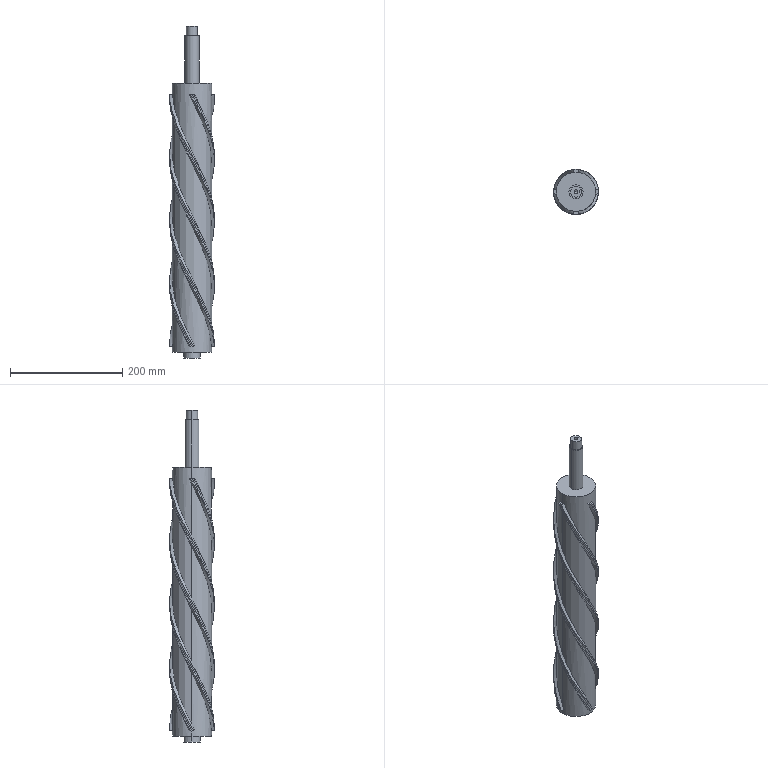Part | SolidWorks | features ICE 4, Extrusion 1, Helix 1, HoleWzd 1, Sweep 1 | 1 solid | 53 faces | box 80.225 x 80.225 x 592.5 mm | volume 1973629 mm3 | cylinder 19 | plane 16 | spline 16 | cone 2 | commonest cylinder face diameters 70 x8 6 x3 6.8 x2 20 x2 25 x2 30 x2